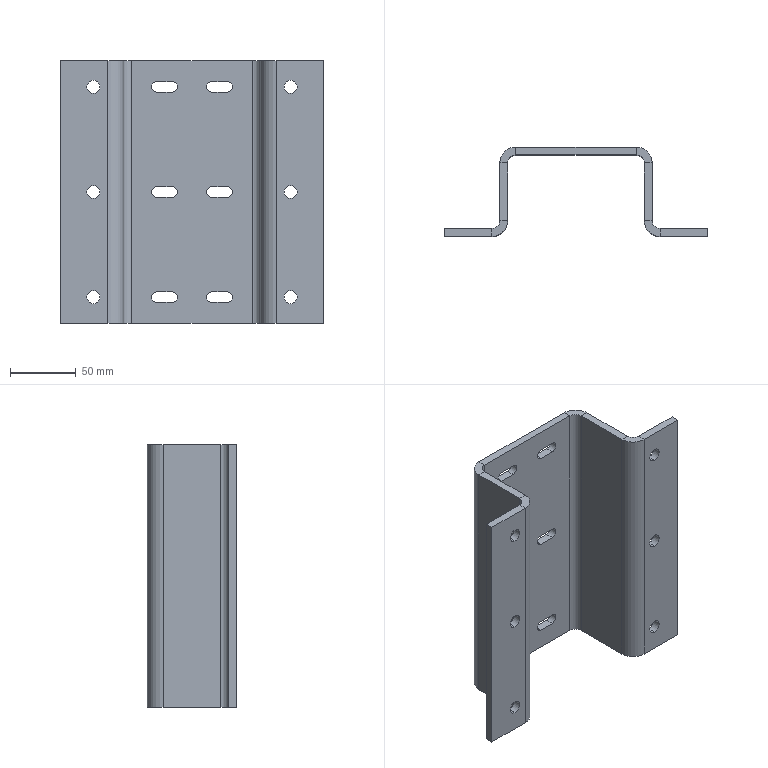Part | STEP file | 01-Gland cover 1 | 1 solid | 74 faces | box 200 x 68 x 200 mm | volume 362165 mm3 | plane 42 | cylinder 32 | commonest cylinder face diameters 8 x12 10 x12 12 x4 24 x4